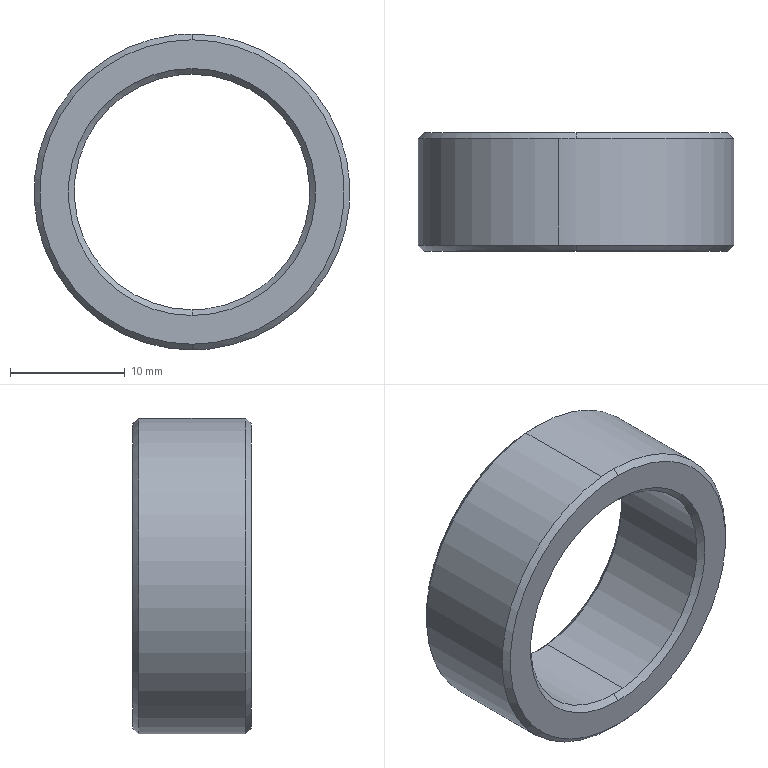Part | SolidWorks | features BaseBody 1 | 1 solid | 14 faces | box 27.5 x 10.3 x 27.5 mm | volume 2680 mm3 | cone 8 | cylinder 4 | plane 2 | commonest cylinder face diameters 20.5 x2 27.5 x2
STEP:
#1=CARTESIAN_POINT('',(-530.322,-97.95,31.541));
#2=VERTEX_POINT('',#1);
#3=CARTESIAN_POINT('',(-530.322,-97.95,5.041));
#4=VERTEX_POINT('',#3);
#5=CARTESIAN_POINT('',(-530.322,-97.95,18.291));
#6=DIRECTION('',(0.,-1.,0.));
#7=DIRECTION('',(0.,0.,-1.));
#8=AXIS2_PLACEMENT_3D('',#5,#6,#7);
#9=CIRCLE('',#8,13.25);
#10=EDGE_CURVE('',#2,#4,#9,.T.);
#11=ORIENTED_EDGE('',*,*,#10,.F.);
#12=CARTESIAN_POINT('',(-530.322,-97.45,32.041));
#13=VERTEX_POINT('',#12);
#14=CARTESIAN_POINT('',(-530.322,-97.95,31.541));
#15=DIRECTION('',(0.,0.7071,0.7071));
#16=VECTOR('',#15,1000.);
#17=LINE('',#14,#16);
#18=EDGE_CURVE('',#2,#13,#17,.T.);
#19=ORIENTED_EDGE('',*,*,#18,.T.);
#20=CARTESIAN_POINT('',(-531.83,-97.45,31.958));
#21=VERTEX_POINT('',#20);
#22=CARTESIAN_POINT('',(-530.322,-97.45,18.291));
#23=DIRECTION('',(0.,1.,0.));
#24=DIRECTION('',(0.,0.,1.));
#25=AXIS2_PLACEMENT_3D('',#22,#23,#24);
#26=CIRCLE('',#25,13.75);
#27=EDGE_CURVE('',#21,#13,#26,.T.);
#28=ORIENTED_EDGE('',*,*,#27,.F.);
#29=CARTESIAN_POINT('',(-530.322,-97.45,4.541));
#30=VERTEX_POINT('',#29);
#31=CARTESIAN_POINT('',(-530.322,-97.45,18.291));
#32=DIRECTION('',(0.,1.,0.));
#33=DIRECTION('',(0.,0.,1.));
#34=AXIS2_PLACEMENT_3D('',#31,#32,#33);
#35=CIRCLE('',#34,13.75);
#36=EDGE_CURVE('',#30,#21,#35,.T.);
#37=ORIENTED_EDGE('',*,*,#36,.F.);
#38=CARTESIAN_POINT('',(-530.322,-97.95,5.041));
#39=DIRECTION('',(0.,0.7071,-0.7071));
#40=VECTOR('',#39,1000.);
#41=LINE('',#38,#40);
#42=EDGE_CURVE('',#4,#30,#41,.T.);
#43=ORIENTED_EDGE('',*,*,#42,.F.);
#44=EDGE_LOOP('',(#11,#19,#28,#37,#43));
#45=FACE_OUTER_BOUND('',#44,.T.);
#46=CARTESIAN_POINT('',(-530.322,-97.95,18.291));
#47=DIRECTION('',(0.,1.,0.));
#48=DIRECTION('',(0.,0.,-1.));
#49=AXIS2_PLACEMENT_3D('',#46,#47,#48);
#50=CONICAL_SURFACE('',#49,13.25,0.7854);
#51=ADVANCED_FACE('',(#45),#50,.T.);
#52=CARTESIAN_POINT('',(-530.322,-97.45,8.041));
#53=VERTEX_POINT('',#52);
#54=CARTESIAN_POINT('',(-529.197,-97.45,8.103));
#55=VERTEX_POINT('',#54);
#56=CARTESIAN_POINT('',(-530.322,-97.45,18.291));
#57=DIRECTION('',(0.,-1.,0.));
#58=DIRECTION('',(0.,0.,-1.));
#59=AXIS2_PLACEMENT_3D('',#56,#57,#58);
#60=CIRCLE('',#59,10.25);
#61=EDGE_CURVE('',#53,#55,#60,.T.);
#62=ORIENTED_EDGE('',*,*,#61,.F.);
#63=CARTESIAN_POINT('',(-530.322,-97.95,7.541));
#64=VERTEX_POINT('',#63);
#65=CARTESIAN_POINT('',(-530.322,-97.45,8.041));
#66=DIRECTION('',(0.,-0.7071,-0.7071));
#67=VECTOR('',#66,1000.);
#68=LINE('',#65,#67);
#69=EDGE_CURVE('',#53,#64,#68,.T.);
#70=ORIENTED_EDGE('',*,*,#69,.T.);
#71=CARTESIAN_POINT('',(-530.322,-97.95,29.041));
#72=VERTEX_POINT('',#71);
#73=CARTESIAN_POINT('',(-530.322,-97.95,18.291));
#74=DIRECTION('',(0.,1.,0.));
#75=DIRECTION('',(0.,0.,-1.));
#76=AXIS2_PLACEMENT_3D('',#73,#74,#75);
#77=CIRCLE('',#76,10.75);
#78=EDGE_CURVE('',#72,#64,#77,.T.);
#79=ORIENTED_EDGE('',*,*,#78,.F.);
#80=CARTESIAN_POINT('',(-530.322,-97.45,28.541));
#81=VERTEX_POINT('',#80);
#82=CARTESIAN_POINT('',(-530.322,-97.45,28.541));
#83=DIRECTION('',(0.,-0.7071,0.7071));
#84=VECTOR('',#83,1000.);
#85=LINE('',#82,#84);
#86=EDGE_CURVE('',#81,#72,#85,.T.);
#87=ORIENTED_EDGE('',*,*,#86,.F.);
#88=CARTESIAN_POINT('',(-530.322,-97.45,18.291));
#89=DIRECTION('',(0.,-1.,0.));
#90=DIRECTION('',(0.,0.,-1.));
#91=AXIS2_PLACEMENT_3D('',#88,#89,#90);
#92=CIRCLE('',#91,10.25);
#93=EDGE_CURVE('',#55,#81,#92,.T.);
#94=ORIENTED_EDGE('',*,*,#93,.F.);
#95=EDGE_LOOP('',(#62,#70,#79,#87,#94));
#96=FACE_OUTER_BOUND('',#95,.T.);
#97=CARTESIAN_POINT('',(-530.322,-97.45,18.291));
#98=DIRECTION('',(0.,-1.,0.));
#99=DIRECTION('',(0.,0.,1.));
#100=AXIS2_PLACEMENT_3D('',#97,#98,#99);
#101=CONICAL_SURFACE('',#100,10.25,0.7854);
#102=ADVANCED_FACE('',(#96),#101,.F.);
#103=CARTESIAN_POINT('',(-530.322,-88.15,28.541));
#104=VERTEX_POINT('',#103);
#105=CARTESIAN_POINT('',(-529.197,-88.15,8.103));
#106=VERTEX_POINT('',#105);
#107=CARTESIAN_POINT('',(-530.322,-88.15,18.291));
#108=DIRECTION('',(0.,1.,0.));
#109=DIRECTION('',(0.,0.,1.));
#110=AXIS2_PLACEMENT_3D('',#107,#108,#109);
#111=CIRCLE('',#110,10.25);
#112=EDGE_CURVE('',#104,#106,#111,.T.);
#113=ORIENTED_EDGE('',*,*,#112,.F.);
#114=CARTESIAN_POINT('',(-530.322,-87.65,29.041));
#115=VERTEX_POINT('',#114);
#116=CARTESIAN_POINT('',(-530.322,-87.65,29.041));
#117=DIRECTION('',(0.,0.7071,0.7071));
#118=VECTOR('',#117,1000.);
#119=LINE('',#116,#118);
#120=EDGE_CURVE('',#104,#115,#119,.T.);
#121=ORIENTED_EDGE('',*,*,#120,.T.);
#122=CARTESIAN_POINT('',(-530.322,-87.65,7.541));
#123=VERTEX_POINT('',#122);
#124=CARTESIAN_POINT('',(-530.322,-87.65,18.291));
#125=DIRECTION('',(0.,-1.,0.));
#126=DIRECTION('',(0.,0.,1.));
#127=AXIS2_PLACEMENT_3D('',#124,#125,#126);
#128=CIRCLE('',#127,10.75);
#129=EDGE_CURVE('',#123,#115,#128,.T.);
#130=ORIENTED_EDGE('',*,*,#129,.F.);
#131=CARTESIAN_POINT('',(-530.322,-88.15,8.041));
#132=VERTEX_POINT('',#131);
#133=CARTESIAN_POINT('',(-530.322,-87.65,7.541));
#134=DIRECTION('',(0.,0.7071,-0.7071));
#135=VECTOR('',#134,1000.);
#136=LINE('',#133,#135);
#137=EDGE_CURVE('',#132,#123,#136,.T.);
#138=ORIENTED_EDGE('',*,*,#137,.F.);
#139=CARTESIAN_POINT('',(-530.322,-88.15,18.291));
#140=DIRECTION('',(0.,1.,0.));
#141=DIRECTION('',(0.,0.,1.));
#142=AXIS2_PLACEMENT_3D('',#139,#140,#141);
#143=CIRCLE('',#142,10.25);
#144=EDGE_CURVE('',#106,#132,#143,.T.);
#145=ORIENTED_EDGE('',*,*,#144,.F.);
#146=EDGE_LOOP('',(#113,#121,#130,#138,#145));
#147=FACE_OUTER_BOUND('',#146,.T.);
#148=CARTESIAN_POINT('',(-530.322,-87.65,18.291));
#149=DIRECTION('',(0.,1.,0.));
#150=DIRECTION('',(0.,0.,-1.));
#151=AXIS2_PLACEMENT_3D('',#148,#149,#150);
#152=CONICAL_SURFACE('',#151,10.75,0.7854);
#153=ADVANCED_FACE('',(#147),#152,.F.);
#154=CARTESIAN_POINT('',(-530.322,-87.65,5.041));
#155=VERTEX_POINT('',#154);
#156=CARTESIAN_POINT('',(-530.322,-87.65,31.541));
#157=VERTEX_POINT('',#156);
#158=CARTESIAN_POINT('',(-530.322,-87.65,18.291));
#159=DIRECTION('',(0.,1.,0.));
#160=DIRECTION('',(0.,0.,1.));
#161=AXIS2_PLACEMENT_3D('',#158,#159,#160);
#162=CIRCLE('',#161,13.25);
#163=EDGE_CURVE('',#155,#157,#162,.T.);
#164=ORIENTED_EDGE('',*,*,#163,.F.);
#165=CARTESIAN_POINT('',(-530.322,-88.15,4.541));
#166=VERTEX_POINT('',#165);
#167=CARTESIAN_POINT('',(-530.322,-88.15,4.541));
#168=DIRECTION('',(0.,-0.7071,-0.7071));
#169=VECTOR('',#168,1000.);
#170=LINE('',#167,#169);
#171=EDGE_CURVE('',#155,#166,#170,.T.);
#172=ORIENTED_EDGE('',*,*,#171,.T.);
#173=CARTESIAN_POINT('',(-531.83,-88.15,31.958));
#174=VERTEX_POINT('',#173);
#175=CARTESIAN_POINT('',(-530.322,-88.15,18.291));
#176=DIRECTION('',(0.,-1.,0.));
#177=DIRECTION('',(0.,0.,-1.));
#178=AXIS2_PLACEMENT_3D('',#175,#176,#177);
#179=CIRCLE('',#178,13.75);
#180=EDGE_CURVE('',#174,#166,#179,.T.);
#181=ORIENTED_EDGE('',*,*,#180,.F.);
#182=CARTESIAN_POINT('',(-530.322,-88.15,32.041));
#183=VERTEX_POINT('',#182);
#184=CARTESIAN_POINT('',(-530.322,-88.15,18.291));
#185=DIRECTION('',(0.,-1.,0.));
#186=DIRECTION('',(0.,0.,-1.));
#187=AXIS2_PLACEMENT_3D('',#184,#185,#186);
#188=CIRCLE('',#187,13.75);
#189=EDGE_CURVE('',#183,#174,#188,.T.);
#190=ORIENTED_EDGE('',*,*,#189,.F.);
#191=CARTESIAN_POINT('',(-530.322,-88.15,32.041));
#192=DIRECTION('',(0.,-0.7071,0.7071));
#193=VECTOR('',#192,1000.);
#194=LINE('',#191,#193);
#195=EDGE_CURVE('',#157,#183,#194,.T.);
#196=ORIENTED_EDGE('',*,*,#195,.F.);
#197=EDGE_LOOP('',(#164,#172,#181,#190,#196));
#198=FACE_OUTER_BOUND('',#197,.T.);
#199=CARTESIAN_POINT('',(-530.322,-88.15,18.291));
#200=DIRECTION('',(0.,-1.,0.));
#201=DIRECTION('',(0.,0.,1.));
#202=AXIS2_PLACEMENT_3D('',#199,#200,#201);
#203=CONICAL_SURFACE('',#202,13.75,0.7854);
#204=ADVANCED_FACE('',(#198),#203,.T.);
#205=CARTESIAN_POINT('',(-531.446,-97.45,28.479));
#206=VERTEX_POINT('',#205);
#207=CARTESIAN_POINT('',(-530.322,-97.45,18.291));
#208=DIRECTION('',(0.,-1.,0.));
#209=DIRECTION('',(0.,0.,-1.));
#210=AXIS2_PLACEMENT_3D('',#207,#208,#209);
#211=CIRCLE('',#210,10.25);
#212=EDGE_CURVE('',#206,#53,#211,.T.);
#213=ORIENTED_EDGE('',*,*,#212,.T.);
#214=ORIENTED_EDGE('',*,*,#61,.T.);
#215=CARTESIAN_POINT('',(-529.197,-102.,8.103));
#216=DIRECTION('',(0.,1.,0.));
#217=VECTOR('',#216,1000.);
#218=LINE('',#215,#217);
#219=EDGE_CURVE('',#55,#106,#218,.T.);
#220=ORIENTED_EDGE('',*,*,#219,.T.);
#221=ORIENTED_EDGE('',*,*,#144,.T.);
#222=CARTESIAN_POINT('',(-531.446,-88.15,28.479));
#223=VERTEX_POINT('',#222);
#224=CARTESIAN_POINT('',(-530.322,-88.15,18.291));
#225=DIRECTION('',(0.,1.,0.));
#226=DIRECTION('',(0.,0.,1.));
#227=AXIS2_PLACEMENT_3D('',#224,#225,#226);
#228=CIRCLE('',#227,10.25);
#229=EDGE_CURVE('',#132,#223,#228,.T.);
#230=ORIENTED_EDGE('',*,*,#229,.T.);
#231=CARTESIAN_POINT('',(-531.446,-102.,28.479));
#232=DIRECTION('',(0.,1.,0.));
#233=VECTOR('',#232,1000.);
#234=LINE('',#231,#233);
#235=EDGE_CURVE('',#206,#223,#234,.T.);
#236=ORIENTED_EDGE('',*,*,#235,.F.);
#237=EDGE_LOOP('',(#213,#214,#220,#221,#230,#236));
#238=FACE_OUTER_BOUND('',#237,.T.);
#239=CARTESIAN_POINT('',(-530.322,-102.,18.291));
#240=DIRECTION('',(0.,1.,0.));
#241=DIRECTION('',(-0.1097,0.,0.994));
#242=AXIS2_PLACEMENT_3D('',#239,#240,#241);
#243=CYLINDRICAL_SURFACE('',#242,10.25);
#244=ADVANCED_FACE('',(#238),#243,.F.);
#245=ORIENTED_EDGE('',*,*,#27,.T.);
#246=CARTESIAN_POINT('',(-528.813,-97.45,4.624));
#247=VERTEX_POINT('',#246);
#248=CARTESIAN_POINT('',(-530.322,-97.45,18.291));
#249=DIRECTION('',(0.,1.,0.));
#250=DIRECTION('',(0.,0.,1.));
#251=AXIS2_PLACEMENT_3D('',#248,#249,#250);
#252=CIRCLE('',#251,13.75);
#253=EDGE_CURVE('',#13,#247,#252,.T.);
#254=ORIENTED_EDGE('',*,*,#253,.T.);
#255=CARTESIAN_POINT('',(-528.813,-88.15,4.624));
#256=VERTEX_POINT('',#255);
#257=CARTESIAN_POINT('',(-528.813,-102.,4.624));
#258=DIRECTION('',(0.,1.,0.));
#259=VECTOR('',#258,1000.);
#260=LINE('',#257,#259);
#261=EDGE_CURVE('',#247,#256,#260,.T.);
#262=ORIENTED_EDGE('',*,*,#261,.T.);
#263=CARTESIAN_POINT('',(-530.322,-88.15,18.291));
#264=DIRECTION('',(0.,-1.,0.));
#265=DIRECTION('',(0.,0.,-1.));
#266=AXIS2_PLACEMENT_3D('',#263,#264,#265);
#267=CIRCLE('',#266,13.75);
#268=EDGE_CURVE('',#256,#183,#267,.T.);
#269=ORIENTED_EDGE('',*,*,#268,.T.);
#270=ORIENTED_EDGE('',*,*,#189,.T.);
#271=CARTESIAN_POINT('',(-531.83,-102.,31.958));
#272=DIRECTION('',(0.,1.,0.));
#273=VECTOR('',#272,1000.);
#274=LINE('',#271,#273);
#275=EDGE_CURVE('',#21,#174,#274,.T.);
#276=ORIENTED_EDGE('',*,*,#275,.F.);
#277=EDGE_LOOP('',(#245,#254,#262,#269,#270,#276));
#278=FACE_OUTER_BOUND('',#277,.T.);
#279=CARTESIAN_POINT('',(-530.322,-102.,18.291));
#280=DIRECTION('',(0.,1.,0.));
#281=DIRECTION('',(-0.1097,0.,0.994));
#282=AXIS2_PLACEMENT_3D('',#279,#280,#281);
#283=CYLINDRICAL_SURFACE('',#282,13.75);
#284=ADVANCED_FACE('',(#278),#283,.T.);
#285=ORIENTED_EDGE('',*,*,#129,.T.);
#286=CARTESIAN_POINT('',(-530.322,-87.65,18.291));
#287=DIRECTION('',(0.,-1.,0.));
#288=DIRECTION('',(0.,0.,1.));
#289=AXIS2_PLACEMENT_3D('',#286,#287,#288);
#290=CIRCLE('',#289,10.75);
#291=EDGE_CURVE('',#115,#123,#290,.T.);
#292=ORIENTED_EDGE('',*,*,#291,.T.);
#293=EDGE_LOOP('',(#285,#292));
#294=FACE_BOUND('',#293,.T.);
#295=CARTESIAN_POINT('',(-530.322,-87.65,18.291));
#296=DIRECTION('',(0.,1.,0.));
#297=DIRECTION('',(0.,0.,1.));
#298=AXIS2_PLACEMENT_3D('',#295,#296,#297);
#299=CIRCLE('',#298,13.25);
#300=EDGE_CURVE('',#157,#155,#299,.T.);
#301=ORIENTED_EDGE('',*,*,#300,.T.);
#302=ORIENTED_EDGE('',*,*,#163,.T.);
#303=EDGE_LOOP('',(#301,#302));
#304=FACE_OUTER_BOUND('',#303,.T.);
#305=CARTESIAN_POINT('',(-530.322,-87.65,18.291));
#306=DIRECTION('',(0.,1.,0.));
#307=DIRECTION('',(1.,0.,0.));
#308=AXIS2_PLACEMENT_3D('',#305,#306,#307);
#309=PLANE('',#308);
#310=ADVANCED_FACE('',(#294,#304),#309,.T.);
#311=ORIENTED_EDGE('',*,*,#261,.F.);
#312=CARTESIAN_POINT('',(-530.322,-97.45,18.291));
#313=DIRECTION('',(0.,1.,0.));
#314=DIRECTION('',(0.,0.,1.));
#315=AXIS2_PLACEMENT_3D('',#312,#313,#314);
#316=CIRCLE('',#315,13.75);
#317=EDGE_CURVE('',#247,#30,#316,.T.);
#318=ORIENTED_EDGE('',*,*,#317,.T.);
#319=ORIENTED_EDGE('',*,*,#36,.T.);
#320=ORIENTED_EDGE('',*,*,#275,.T.);
#321=ORIENTED_EDGE('',*,*,#180,.T.);
#322=CARTESIAN_POINT('',(-530.322,-88.15,18.291));
#323=DIRECTION('',(0.,-1.,0.));
#324=DIRECTION('',(0.,0.,-1.));
#325=AXIS2_PLACEMENT_3D('',#322,#323,#324);
#326=CIRCLE('',#325,13.75);
#327=EDGE_CURVE('',#166,#256,#326,.T.);
#328=ORIENTED_EDGE('',*,*,#327,.T.);
#329=EDGE_LOOP('',(#311,#318,#319,#320,#321,#328));
#330=FACE_OUTER_BOUND('',#329,.T.);
#331=CARTESIAN_POINT('',(-530.322,-102.,18.291));
#332=DIRECTION('',(0.,1.,0.));
#333=DIRECTION('',(-0.1097,0.,0.994));
#334=AXIS2_PLACEMENT_3D('',#331,#332,#333);
#335=CYLINDRICAL_SURFACE('',#334,13.75);
#336=ADVANCED_FACE('',(#330),#335,.T.);
#337=ORIENTED_EDGE('',*,*,#219,.F.);
#338=ORIENTED_EDGE('',*,*,#93,.T.);
#339=CARTESIAN_POINT('',(-530.322,-97.45,18.291));
#340=DIRECTION('',(0.,-1.,0.));
#341=DIRECTION('',(0.,0.,-1.));
#342=AXIS2_PLACEMENT_3D('',#339,#340,#341);
#343=CIRCLE('',#342,10.25);
#344=EDGE_CURVE('',#81,#206,#343,.T.);
#345=ORIENTED_EDGE('',*,*,#344,.T.);
#346=ORIENTED_EDGE('',*,*,#235,.T.);
#347=CARTESIAN_POINT('',(-530.322,-88.15,18.291));
#348=DIRECTION('',(0.,1.,0.));
#349=DIRECTION('',(0.,0.,1.));
#350=AXIS2_PLACEMENT_3D('',#347,#348,#349);
#351=CIRCLE('',#350,10.25);
#352=EDGE_CURVE('',#223,#104,#351,.T.);
#353=ORIENTED_EDGE('',*,*,#352,.T.);
#354=ORIENTED_EDGE('',*,*,#112,.T.);
#355=EDGE_LOOP('',(#337,#338,#345,#346,#353,#354));
#356=FACE_OUTER_BOUND('',#355,.T.);
#357=CARTESIAN_POINT('',(-530.322,-102.,18.291));
#358=DIRECTION('',(0.,1.,0.));
#359=DIRECTION('',(-0.1097,0.,0.994));
#360=AXIS2_PLACEMENT_3D('',#357,#358,#359);
#361=CYLINDRICAL_SURFACE('',#360,10.25);
#362=ADVANCED_FACE('',(#356),#361,.F.);
#363=ORIENTED_EDGE('',*,*,#78,.T.);
#364=CARTESIAN_POINT('',(-530.322,-97.95,18.291));
#365=DIRECTION('',(0.,1.,0.));
#366=DIRECTION('',(0.,0.,-1.));
#367=AXIS2_PLACEMENT_3D('',#364,#365,#366);
#368=CIRCLE('',#367,10.75);
#369=EDGE_CURVE('',#64,#72,#368,.T.);
#370=ORIENTED_EDGE('',*,*,#369,.T.);
#371=EDGE_LOOP('',(#363,#370));
#372=FACE_BOUND('',#371,.T.);
#373=CARTESIAN_POINT('',(-530.322,-97.95,18.291));
#374=DIRECTION('',(0.,-1.,0.));
#375=DIRECTION('',(0.,0.,-1.));
#376=AXIS2_PLACEMENT_3D('',#373,#374,#375);
#377=CIRCLE('',#376,13.25);
#378=EDGE_CURVE('',#4,#2,#377,.T.);
#379=ORIENTED_EDGE('',*,*,#378,.T.);
#380=ORIENTED_EDGE('',*,*,#10,.T.);
#381=EDGE_LOOP('',(#379,#380));
#382=FACE_OUTER_BOUND('',#381,.T.);
#383=CARTESIAN_POINT('',(-530.322,-97.95,18.291));
#384=DIRECTION('',(0.,-1.,0.));
#385=DIRECTION('',(0.,0.,-1.));
#386=AXIS2_PLACEMENT_3D('',#383,#384,#385);
#387=PLANE('',#386);
#388=ADVANCED_FACE('',(#372,#382),#387,.T.);
#389=ORIENTED_EDGE('',*,*,#171,.F.);
#390=ORIENTED_EDGE('',*,*,#300,.F.);
#391=ORIENTED_EDGE('',*,*,#195,.T.);
#392=ORIENTED_EDGE('',*,*,#268,.F.);
#393=ORIENTED_EDGE('',*,*,#327,.F.);
#394=EDGE_LOOP('',(#389,#390,#391,#392,#393));
#395=FACE_OUTER_BOUND('',#394,.T.);
#396=CARTESIAN_POINT('',(-530.322,-88.15,18.291));
#397=DIRECTION('',(0.,-1.,0.));
#398=DIRECTION('',(0.,0.,1.));
#399=AXIS2_PLACEMENT_3D('',#396,#397,#398);
#400=CONICAL_SURFACE('',#399,13.75,0.7854);
#401=ADVANCED_FACE('',(#395),#400,.T.);
#402=ORIENTED_EDGE('',*,*,#120,.F.);
#403=ORIENTED_EDGE('',*,*,#352,.F.);
#404=ORIENTED_EDGE('',*,*,#229,.F.);
#405=ORIENTED_EDGE('',*,*,#137,.T.);
#406=ORIENTED_EDGE('',*,*,#291,.F.);
#407=EDGE_LOOP('',(#402,#403,#404,#405,#406));
#408=FACE_OUTER_BOUND('',#407,.T.);
#409=CARTESIAN_POINT('',(-530.322,-87.65,18.291));
#410=DIRECTION('',(0.,1.,0.));
#411=DIRECTION('',(0.,0.,-1.));
#412=AXIS2_PLACEMENT_3D('',#409,#410,#411);
#413=CONICAL_SURFACE('',#412,10.75,0.7854);
#414=ADVANCED_FACE('',(#408),#413,.F.);
#415=ORIENTED_EDGE('',*,*,#69,.F.);
#416=ORIENTED_EDGE('',*,*,#212,.F.);
#417=ORIENTED_EDGE('',*,*,#344,.F.);
#418=ORIENTED_EDGE('',*,*,#86,.T.);
#419=ORIENTED_EDGE('',*,*,#369,.F.);
#420=EDGE_LOOP('',(#415,#416,#417,#418,#419));
#421=FACE_OUTER_BOUND('',#420,.T.);
#422=CARTESIAN_POINT('',(-530.322,-97.45,18.291));
#423=DIRECTION('',(0.,-1.,0.));
#424=DIRECTION('',(0.,0.,1.));
#425=AXIS2_PLACEMENT_3D('',#422,#423,#424);
#426=CONICAL_SURFACE('',#425,10.25,0.7854);
#427=ADVANCED_FACE('',(#421),#426,.F.);
#428=ORIENTED_EDGE('',*,*,#18,.F.);
#429=ORIENTED_EDGE('',*,*,#378,.F.);
#430=ORIENTED_EDGE('',*,*,#42,.T.);
#431=ORIENTED_EDGE('',*,*,#317,.F.);
#432=ORIENTED_EDGE('',*,*,#253,.F.);
#433=EDGE_LOOP('',(#428,#429,#430,#431,#432));
#434=FACE_OUTER_BOUND('',#433,.T.);
#435=CARTESIAN_POINT('',(-530.322,-97.95,18.291));
#436=DIRECTION('',(0.,1.,0.));
#437=DIRECTION('',(0.,0.,-1.));
#438=AXIS2_PLACEMENT_3D('',#435,#436,#437);
#439=CONICAL_SURFACE('',#438,13.25,0.7854);
#440=ADVANCED_FACE('',(#434),#439,.T.);
#441=CLOSED_SHELL('',(#51,#102,#153,#204,#244,#284,#310,#336,#362,#388,#401,#414,#427,#440));
#442=MANIFOLD_SOLID_BREP('',#441);
#443=CARTESIAN_POINT('',(0.,0.,0.));
#444=DIRECTION('',(0.,0.,1.));
#445=DIRECTION('',(1.,0.,0.));
#446=AXIS2_PLACEMENT_3D('',#443,#444,#445);
#447=(LENGTH_UNIT()NAMED_UNIT(*)SI_UNIT(.MILLI.,.METRE.));
#448=UNCERTAINTY_MEASURE_WITH_UNIT(LENGTH_MEASURE(0.00001),#447,'','');
#449=(NAMED_UNIT(*)PLANE_ANGLE_UNIT()SI_UNIT($,.RADIAN.));
#450=(NAMED_UNIT(*)SI_UNIT($,.STERADIAN.)SOLID_ANGLE_UNIT());
#451=(GEOMETRIC_REPRESENTATION_CONTEXT(3)GLOBAL_UNCERTAINTY_ASSIGNED_CONTEXT((#448))GLOBAL_UNIT_ASSIGNED_CONTEXT((#447,#449,#450))REPRESENTATION_CONTEXT('',''));
#452=ADVANCED_BREP_SHAPE_REPRESENTATION('',(#442,#446),#451);